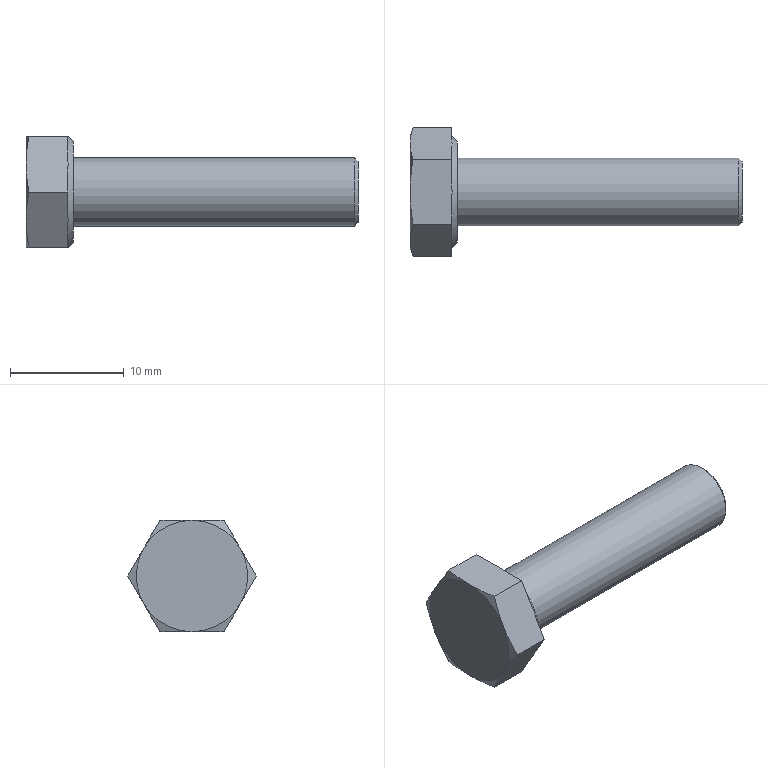Part | STEP file | Hex head bolt M6X25 A2-70 GBT5783-2016_GB_FASTENER_BOLT_STBAB A M6X25-N | 1 solid | 24 faces | box 29.15 x 11.293 x 9.78 mm | volume 1042 mm3 | plane 15 | cone 8 | cylinder 1 | commonest cylinder face diameters 6 x1